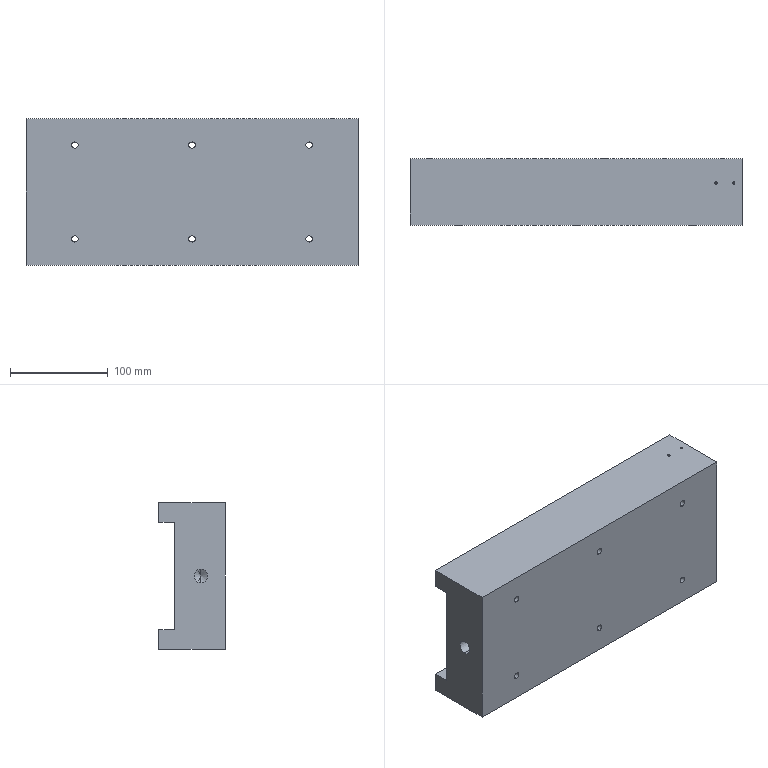Part | NX | features BREP 1 | 1 solid | 168 faces | box 340 x 68 x 150 mm | volume 2833787 mm3 | cylinder 88 | cone 64 | plane 16 | commonest cylinder face diameters 3.3 x56 6.6 x12 13 x12 2.5 x4 14 x4